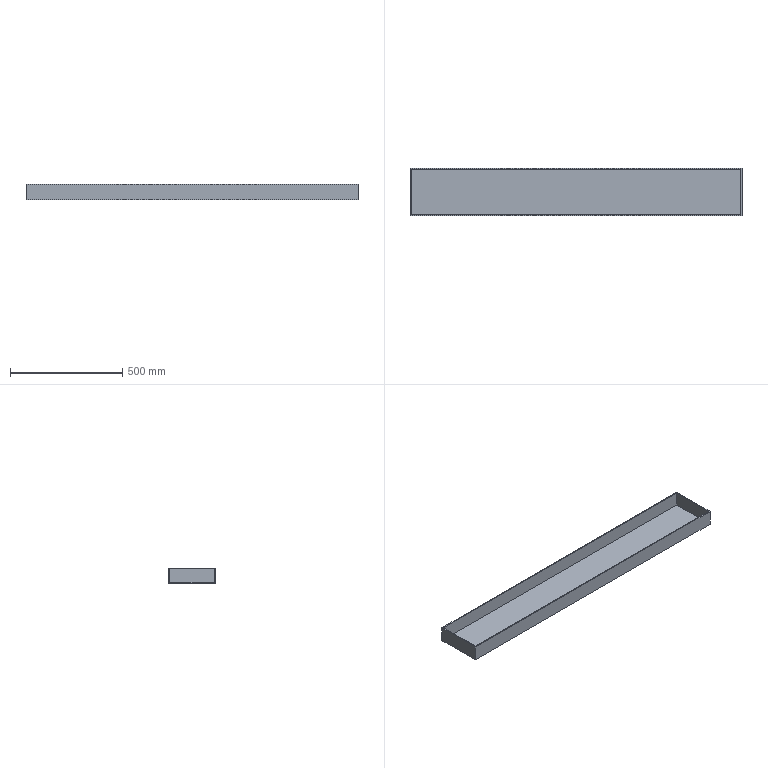Part | SolidWorks | features ExtruThin 1, ICE 1 | 1 solid | 11 faces | box 1480 x 210 x 70 mm | volume 2646000 mm3 | plane 11
STEP:
#1=CARTESIAN_POINT('',(735.,100.,70.));
#2=VERTEX_POINT('',#1);
#3=CARTESIAN_POINT('',(735.,100.,5.));
#4=VERTEX_POINT('',#3);
#5=CARTESIAN_POINT('',(735.,100.,70.));
#6=DIRECTION('',(0.,0.,-1.));
#7=VECTOR('',#6,1000.);
#8=LINE('',#5,#7);
#9=EDGE_CURVE('',#2,#4,#8,.T.);
#10=ORIENTED_EDGE('',*,*,#9,.T.);
#11=CARTESIAN_POINT('',(735.,-100.,5.));
#12=VERTEX_POINT('',#11);
#13=CARTESIAN_POINT('',(735.,105.,5.));
#14=DIRECTION('',(0.,1.,0.));
#15=VECTOR('',#14,1000.);
#16=LINE('',#13,#15);
#17=EDGE_CURVE('',#12,#4,#16,.T.);
#18=ORIENTED_EDGE('',*,*,#17,.F.);
#19=CARTESIAN_POINT('',(735.,-100.,70.));
#20=VERTEX_POINT('',#19);
#21=CARTESIAN_POINT('',(735.,-100.,70.));
#22=DIRECTION('',(0.,0.,-1.));
#23=VECTOR('',#22,1000.);
#24=LINE('',#21,#23);
#25=EDGE_CURVE('',#20,#12,#24,.T.);
#26=ORIENTED_EDGE('',*,*,#25,.F.);
#27=CARTESIAN_POINT('',(735.,-100.,70.));
#28=DIRECTION('',(0.,1.,0.));
#29=VECTOR('',#28,1000.);
#30=LINE('',#27,#29);
#31=EDGE_CURVE('',#20,#2,#30,.T.);
#32=ORIENTED_EDGE('',*,*,#31,.T.);
#33=EDGE_LOOP('',(#10,#18,#26,#32));
#34=FACE_OUTER_BOUND('',#33,.T.);
#35=CARTESIAN_POINT('',(735.,-100.,70.));
#36=DIRECTION('',(-1.,0.,0.));
#37=DIRECTION('',(0.,0.,1.));
#38=AXIS2_PLACEMENT_3D('',#35,#36,#37);
#39=PLANE('',#38);
#40=ADVANCED_FACE('',(#34),#39,.T.);
#41=CARTESIAN_POINT('',(-735.,100.,70.));
#42=VERTEX_POINT('',#41);
#43=CARTESIAN_POINT('',(-735.,100.,5.));
#44=VERTEX_POINT('',#43);
#45=CARTESIAN_POINT('',(-735.,100.,70.));
#46=DIRECTION('',(0.,0.,-1.));
#47=VECTOR('',#46,1000.);
#48=LINE('',#45,#47);
#49=EDGE_CURVE('',#42,#44,#48,.T.);
#50=ORIENTED_EDGE('',*,*,#49,.T.);
#51=CARTESIAN_POINT('',(-735.,100.,5.));
#52=DIRECTION('',(1.,0.,0.));
#53=VECTOR('',#52,1000.);
#54=LINE('',#51,#53);
#55=EDGE_CURVE('',#44,#4,#54,.T.);
#56=ORIENTED_EDGE('',*,*,#55,.T.);
#57=ORIENTED_EDGE('',*,*,#9,.F.);
#58=CARTESIAN_POINT('',(-735.,100.,70.));
#59=DIRECTION('',(-1.,0.,0.));
#60=VECTOR('',#59,1000.);
#61=LINE('',#58,#60);
#62=EDGE_CURVE('',#2,#42,#61,.T.);
#63=ORIENTED_EDGE('',*,*,#62,.T.);
#64=EDGE_LOOP('',(#50,#56,#57,#63));
#65=FACE_OUTER_BOUND('',#64,.T.);
#66=CARTESIAN_POINT('',(-735.,100.,70.));
#67=DIRECTION('',(0.,-1.,0.));
#68=DIRECTION('',(0.,0.,-1.));
#69=AXIS2_PLACEMENT_3D('',#66,#67,#68);
#70=PLANE('',#69);
#71=ADVANCED_FACE('',(#65),#70,.T.);
#72=CARTESIAN_POINT('',(-735.,-100.,70.));
#73=VERTEX_POINT('',#72);
#74=CARTESIAN_POINT('',(-735.,-100.,5.));
#75=VERTEX_POINT('',#74);
#76=CARTESIAN_POINT('',(-735.,-100.,70.));
#77=DIRECTION('',(0.,0.,-1.));
#78=VECTOR('',#77,1000.);
#79=LINE('',#76,#78);
#80=EDGE_CURVE('',#73,#75,#79,.T.);
#81=ORIENTED_EDGE('',*,*,#80,.T.);
#82=CARTESIAN_POINT('',(-735.,105.,5.));
#83=DIRECTION('',(0.,-1.,0.));
#84=VECTOR('',#83,1000.);
#85=LINE('',#82,#84);
#86=EDGE_CURVE('',#44,#75,#85,.T.);
#87=ORIENTED_EDGE('',*,*,#86,.F.);
#88=ORIENTED_EDGE('',*,*,#49,.F.);
#89=CARTESIAN_POINT('',(-735.,-100.,70.));
#90=DIRECTION('',(0.,-1.,0.));
#91=VECTOR('',#90,1000.);
#92=LINE('',#89,#91);
#93=EDGE_CURVE('',#42,#73,#92,.T.);
#94=ORIENTED_EDGE('',*,*,#93,.T.);
#95=EDGE_LOOP('',(#81,#87,#88,#94));
#96=FACE_OUTER_BOUND('',#95,.T.);
#97=CARTESIAN_POINT('',(-735.,-100.,70.));
#98=DIRECTION('',(1.,0.,0.));
#99=DIRECTION('',(0.,0.,-1.));
#100=AXIS2_PLACEMENT_3D('',#97,#98,#99);
#101=PLANE('',#100);
#102=ADVANCED_FACE('',(#96),#101,.T.);
#103=ORIENTED_EDGE('',*,*,#25,.T.);
#104=CARTESIAN_POINT('',(-735.,-100.,5.));
#105=DIRECTION('',(-1.,0.,0.));
#106=VECTOR('',#105,1000.);
#107=LINE('',#104,#106);
#108=EDGE_CURVE('',#12,#75,#107,.T.);
#109=ORIENTED_EDGE('',*,*,#108,.T.);
#110=ORIENTED_EDGE('',*,*,#80,.F.);
#111=CARTESIAN_POINT('',(-735.,-100.,70.));
#112=DIRECTION('',(1.,0.,0.));
#113=VECTOR('',#112,1000.);
#114=LINE('',#111,#113);
#115=EDGE_CURVE('',#73,#20,#114,.T.);
#116=ORIENTED_EDGE('',*,*,#115,.T.);
#117=EDGE_LOOP('',(#103,#109,#110,#116));
#118=FACE_OUTER_BOUND('',#117,.T.);
#119=CARTESIAN_POINT('',(-735.,-100.,70.));
#120=DIRECTION('',(0.,1.,0.));
#121=DIRECTION('',(0.,0.,1.));
#122=AXIS2_PLACEMENT_3D('',#119,#120,#121);
#123=PLANE('',#122);
#124=ADVANCED_FACE('',(#118),#123,.T.);
#125=CARTESIAN_POINT('',(740.,-105.,70.));
#126=VERTEX_POINT('',#125);
#127=CARTESIAN_POINT('',(740.,105.,70.));
#128=VERTEX_POINT('',#127);
#129=CARTESIAN_POINT('',(740.,0.,70.));
#130=DIRECTION('',(0.,1.,0.));
#131=VECTOR('',#130,1000.);
#132=LINE('',#129,#131);
#133=EDGE_CURVE('',#126,#128,#132,.T.);
#134=ORIENTED_EDGE('',*,*,#133,.T.);
#135=CARTESIAN_POINT('',(-740.,105.,70.));
#136=VERTEX_POINT('',#135);
#137=CARTESIAN_POINT('',(0.,105.,70.));
#138=DIRECTION('',(-1.,0.,0.));
#139=VECTOR('',#138,1000.);
#140=LINE('',#137,#139);
#141=EDGE_CURVE('',#128,#136,#140,.T.);
#142=ORIENTED_EDGE('',*,*,#141,.T.);
#143=CARTESIAN_POINT('',(-740.,-105.,70.));
#144=VERTEX_POINT('',#143);
#145=CARTESIAN_POINT('',(-740.,0.,70.));
#146=DIRECTION('',(0.,-1.,0.));
#147=VECTOR('',#146,1000.);
#148=LINE('',#145,#147);
#149=EDGE_CURVE('',#136,#144,#148,.T.);
#150=ORIENTED_EDGE('',*,*,#149,.T.);
#151=CARTESIAN_POINT('',(0.,-105.,70.));
#152=DIRECTION('',(1.,0.,0.));
#153=VECTOR('',#152,1000.);
#154=LINE('',#151,#153);
#155=EDGE_CURVE('',#144,#126,#154,.T.);
#156=ORIENTED_EDGE('',*,*,#155,.T.);
#157=EDGE_LOOP('',(#134,#142,#150,#156));
#158=FACE_OUTER_BOUND('',#157,.T.);
#159=ORIENTED_EDGE('',*,*,#62,.F.);
#160=ORIENTED_EDGE('',*,*,#31,.F.);
#161=ORIENTED_EDGE('',*,*,#115,.F.);
#162=ORIENTED_EDGE('',*,*,#93,.F.);
#163=EDGE_LOOP('',(#159,#160,#161,#162));
#164=FACE_BOUND('',#163,.T.);
#165=CARTESIAN_POINT('',(0.,0.,70.));
#166=DIRECTION('',(0.,0.,1.));
#167=DIRECTION('',(1.,0.,0.));
#168=AXIS2_PLACEMENT_3D('',#165,#166,#167);
#169=PLANE('',#168);
#170=ADVANCED_FACE('',(#158,#164),#169,.T.);
#171=CARTESIAN_POINT('',(740.,-105.,0.));
#172=VERTEX_POINT('',#171);
#173=CARTESIAN_POINT('',(740.,105.,0.));
#174=VERTEX_POINT('',#173);
#175=CARTESIAN_POINT('',(740.,0.,0.));
#176=DIRECTION('',(0.,1.,0.));
#177=VECTOR('',#176,1000.);
#178=LINE('',#175,#177);
#179=EDGE_CURVE('',#172,#174,#178,.T.);
#180=ORIENTED_EDGE('',*,*,#179,.F.);
#181=CARTESIAN_POINT('',(-740.,-105.,0.));
#182=VERTEX_POINT('',#181);
#183=CARTESIAN_POINT('',(0.,-105.,0.));
#184=DIRECTION('',(1.,0.,0.));
#185=VECTOR('',#184,1000.);
#186=LINE('',#183,#185);
#187=EDGE_CURVE('',#182,#172,#186,.T.);
#188=ORIENTED_EDGE('',*,*,#187,.F.);
#189=CARTESIAN_POINT('',(-740.,105.,0.));
#190=VERTEX_POINT('',#189);
#191=CARTESIAN_POINT('',(-740.,0.,0.));
#192=DIRECTION('',(0.,-1.,0.));
#193=VECTOR('',#192,1000.);
#194=LINE('',#191,#193);
#195=EDGE_CURVE('',#190,#182,#194,.T.);
#196=ORIENTED_EDGE('',*,*,#195,.F.);
#197=CARTESIAN_POINT('',(0.,105.,0.));
#198=DIRECTION('',(-1.,0.,0.));
#199=VECTOR('',#198,1000.);
#200=LINE('',#197,#199);
#201=EDGE_CURVE('',#174,#190,#200,.T.);
#202=ORIENTED_EDGE('',*,*,#201,.F.);
#203=EDGE_LOOP('',(#180,#188,#196,#202));
#204=FACE_OUTER_BOUND('',#203,.T.);
#205=CARTESIAN_POINT('',(0.,0.,0.));
#206=DIRECTION('',(0.,0.,1.));
#207=DIRECTION('',(1.,0.,0.));
#208=AXIS2_PLACEMENT_3D('',#205,#206,#207);
#209=PLANE('',#208);
#210=ADVANCED_FACE('',(#204),#209,.F.);
#211=ORIENTED_EDGE('',*,*,#179,.T.);
#212=CARTESIAN_POINT('',(740.,105.,70.));
#213=DIRECTION('',(0.,0.,-1.));
#214=VECTOR('',#213,1000.);
#215=LINE('',#212,#214);
#216=EDGE_CURVE('',#128,#174,#215,.T.);
#217=ORIENTED_EDGE('',*,*,#216,.F.);
#218=ORIENTED_EDGE('',*,*,#133,.F.);
#219=CARTESIAN_POINT('',(740.,-105.,70.));
#220=DIRECTION('',(0.,0.,-1.));
#221=VECTOR('',#220,1000.);
#222=LINE('',#219,#221);
#223=EDGE_CURVE('',#126,#172,#222,.T.);
#224=ORIENTED_EDGE('',*,*,#223,.T.);
#225=EDGE_LOOP('',(#211,#217,#218,#224));
#226=FACE_OUTER_BOUND('',#225,.T.);
#227=CARTESIAN_POINT('',(740.,0.,70.));
#228=DIRECTION('',(-1.,0.,0.));
#229=DIRECTION('',(0.,0.,1.));
#230=AXIS2_PLACEMENT_3D('',#227,#228,#229);
#231=PLANE('',#230);
#232=ADVANCED_FACE('',(#226),#231,.F.);
#233=ORIENTED_EDGE('',*,*,#201,.T.);
#234=CARTESIAN_POINT('',(-740.,105.,70.));
#235=DIRECTION('',(0.,0.,-1.));
#236=VECTOR('',#235,1000.);
#237=LINE('',#234,#236);
#238=EDGE_CURVE('',#136,#190,#237,.T.);
#239=ORIENTED_EDGE('',*,*,#238,.F.);
#240=ORIENTED_EDGE('',*,*,#141,.F.);
#241=ORIENTED_EDGE('',*,*,#216,.T.);
#242=EDGE_LOOP('',(#233,#239,#240,#241));
#243=FACE_OUTER_BOUND('',#242,.T.);
#244=CARTESIAN_POINT('',(0.,105.,70.));
#245=DIRECTION('',(0.,-1.,0.));
#246=DIRECTION('',(0.,0.,-1.));
#247=AXIS2_PLACEMENT_3D('',#244,#245,#246);
#248=PLANE('',#247);
#249=ADVANCED_FACE('',(#243),#248,.F.);
#250=ORIENTED_EDGE('',*,*,#195,.T.);
#251=CARTESIAN_POINT('',(-740.,-105.,70.));
#252=DIRECTION('',(0.,0.,-1.));
#253=VECTOR('',#252,1000.);
#254=LINE('',#251,#253);
#255=EDGE_CURVE('',#144,#182,#254,.T.);
#256=ORIENTED_EDGE('',*,*,#255,.F.);
#257=ORIENTED_EDGE('',*,*,#149,.F.);
#258=ORIENTED_EDGE('',*,*,#238,.T.);
#259=EDGE_LOOP('',(#250,#256,#257,#258));
#260=FACE_OUTER_BOUND('',#259,.T.);
#261=CARTESIAN_POINT('',(-740.,0.,70.));
#262=DIRECTION('',(1.,0.,0.));
#263=DIRECTION('',(0.,0.,-1.));
#264=AXIS2_PLACEMENT_3D('',#261,#262,#263);
#265=PLANE('',#264);
#266=ADVANCED_FACE('',(#260),#265,.F.);
#267=ORIENTED_EDGE('',*,*,#187,.T.);
#268=ORIENTED_EDGE('',*,*,#223,.F.);
#269=ORIENTED_EDGE('',*,*,#155,.F.);
#270=ORIENTED_EDGE('',*,*,#255,.T.);
#271=EDGE_LOOP('',(#267,#268,#269,#270));
#272=FACE_OUTER_BOUND('',#271,.T.);
#273=CARTESIAN_POINT('',(0.,-105.,70.));
#274=DIRECTION('',(0.,1.,0.));
#275=DIRECTION('',(0.,0.,1.));
#276=AXIS2_PLACEMENT_3D('',#273,#274,#275);
#277=PLANE('',#276);
#278=ADVANCED_FACE('',(#272),#277,.F.);
#279=ORIENTED_EDGE('',*,*,#55,.F.);
#280=ORIENTED_EDGE('',*,*,#86,.T.);
#281=ORIENTED_EDGE('',*,*,#108,.F.);
#282=ORIENTED_EDGE('',*,*,#17,.T.);
#283=EDGE_LOOP('',(#279,#280,#281,#282));
#284=FACE_OUTER_BOUND('',#283,.T.);
#285=CARTESIAN_POINT('',(-945.06,105.,5.));
#286=DIRECTION('',(0.,0.,-1.));
#287=DIRECTION('',(0.,1.,0.));
#288=AXIS2_PLACEMENT_3D('',#285,#286,#287);
#289=PLANE('',#288);
#290=ADVANCED_FACE('',(#284),#289,.F.);
#291=CLOSED_SHELL('',(#40,#71,#102,#124,#170,#210,#232,#249,#266,#278,#290));
#292=MANIFOLD_SOLID_BREP('',#291);
#293=CARTESIAN_POINT('',(0.,0.,0.));
#294=DIRECTION('',(0.,0.,1.));
#295=DIRECTION('',(1.,0.,0.));
#296=AXIS2_PLACEMENT_3D('',#293,#294,#295);
#297=(LENGTH_UNIT()NAMED_UNIT(*)SI_UNIT(.MILLI.,.METRE.));
#298=UNCERTAINTY_MEASURE_WITH_UNIT(LENGTH_MEASURE(0.00001),#297,'','');
#299=(NAMED_UNIT(*)PLANE_ANGLE_UNIT()SI_UNIT($,.RADIAN.));
#300=(NAMED_UNIT(*)SI_UNIT($,.STERADIAN.)SOLID_ANGLE_UNIT());
#301=(GEOMETRIC_REPRESENTATION_CONTEXT(3)GLOBAL_UNCERTAINTY_ASSIGNED_CONTEXT((#298))GLOBAL_UNIT_ASSIGNED_CONTEXT((#297,#299,#300))REPRESENTATION_CONTEXT('',''));
#302=ADVANCED_BREP_SHAPE_REPRESENTATION('',(#292,#296),#301);